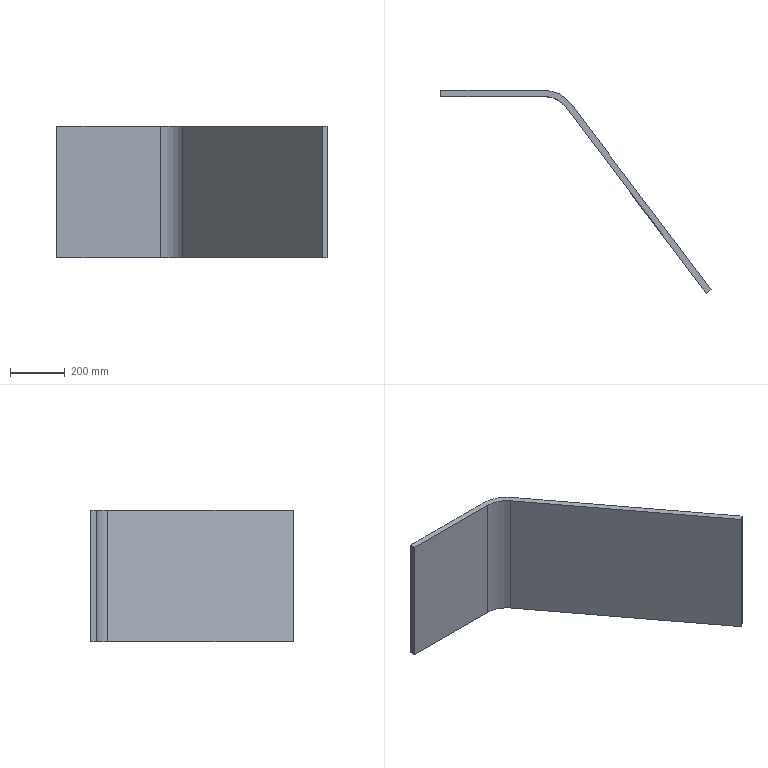Part | NX | features 底座(默认<按焊接>) 2 | 1 solid | 10 faces | box 988.426 x 741.88 x 480 mm | volume 13960123 mm3 | plane 8 | cylinder 2 | commonest cylinder face diameters 200 x1 243.64 x1
STEP:
#1=CARTESIAN_POINT('',(2564.611,34.952,-412.));
#2=VERTEX_POINT('',#1);
#3=CARTESIAN_POINT('',(2052.013,715.193,-412.));
#4=VERTEX_POINT('',#3);
#5=CARTESIAN_POINT('',(3246.385,-869.792,-412.));
#6=DIRECTION('',(-0.6018,0.7986,0.));
#7=VECTOR('',#6,1000.);
#8=LINE('',#5,#7);
#9=EDGE_CURVE('',#2,#4,#8,.T.);
#10=ORIENTED_EDGE('',*,*,#9,.F.);
#11=CARTESIAN_POINT('',(2564.611,34.952,-892.));
#12=VERTEX_POINT('',#11);
#13=CARTESIAN_POINT('',(2564.611,34.952,-892.));
#14=DIRECTION('',(0.,0.,1.));
#15=VECTOR('',#14,1000.);
#16=LINE('',#13,#15);
#17=EDGE_CURVE('',#12,#2,#16,.T.);
#18=ORIENTED_EDGE('',*,*,#17,.F.);
#19=CARTESIAN_POINT('',(2052.013,715.193,-892.));
#20=VERTEX_POINT('',#19);
#21=CARTESIAN_POINT('',(3246.385,-869.792,-892.));
#22=DIRECTION('',(-0.6018,0.7986,0.));
#23=VECTOR('',#22,1000.);
#24=LINE('',#21,#23);
#25=EDGE_CURVE('',#12,#20,#24,.T.);
#26=ORIENTED_EDGE('',*,*,#25,.T.);
#27=CARTESIAN_POINT('',(2052.013,715.193,-892.));
#28=DIRECTION('',(0.,0.,1.));
#29=VECTOR('',#28,1000.);
#30=LINE('',#27,#29);
#31=EDGE_CURVE('',#20,#4,#30,.T.);
#32=ORIENTED_EDGE('',*,*,#31,.T.);
#33=EDGE_LOOP('',(#10,#18,#26,#32));
#34=FACE_BOUND('',#33,.T.);
#35=CARTESIAN_POINT('',(3246.385,-869.792,-892.));
#36=DIRECTION('',(-0.7986,-0.6018,0.));
#37=DIRECTION('',(0.6018,-0.7986,0.));
#38=AXIS2_PLACEMENT_3D('',#35,#36,#37);
#39=PLANE('',#38);
#40=ADVANCED_FACE('',(#34),#39,.F.);
#41=CARTESIAN_POINT('',(1954.723,763.7,-412.));
#42=VERTEX_POINT('',#41);
#43=CARTESIAN_POINT('',(1954.723,641.88,-412.));
#44=DIRECTION('',(0.,0.,1.));
#45=DIRECTION('',(1.,0.,0.));
#46=AXIS2_PLACEMENT_3D('',#43,#44,#45);
#47=CIRCLE('',#46,121.82);
#48=EDGE_CURVE('',#4,#42,#47,.T.);
#49=ORIENTED_EDGE('',*,*,#48,.F.);
#50=ORIENTED_EDGE('',*,*,#31,.F.);
#51=CARTESIAN_POINT('',(1954.723,763.7,-892.));
#52=VERTEX_POINT('',#51);
#53=CARTESIAN_POINT('',(1954.723,641.88,-892.));
#54=DIRECTION('',(0.,0.,1.));
#55=DIRECTION('',(1.,0.,0.));
#56=AXIS2_PLACEMENT_3D('',#53,#54,#55);
#57=CIRCLE('',#56,121.82);
#58=EDGE_CURVE('',#20,#52,#57,.T.);
#59=ORIENTED_EDGE('',*,*,#58,.T.);
#60=CARTESIAN_POINT('',(1954.723,763.7,-892.));
#61=DIRECTION('',(0.,0.,1.));
#62=VECTOR('',#61,1000.);
#63=LINE('',#60,#62);
#64=EDGE_CURVE('',#52,#42,#63,.T.);
#65=ORIENTED_EDGE('',*,*,#64,.T.);
#66=EDGE_LOOP('',(#49,#50,#59,#65));
#67=FACE_BOUND('',#66,.T.);
#68=CARTESIAN_POINT('',(1954.723,641.88,-892.));
#69=DIRECTION('',(0.,0.,1.));
#70=DIRECTION('',(-1.,0.,0.));
#71=AXIS2_PLACEMENT_3D('',#68,#69,#70);
#72=CYLINDRICAL_SURFACE('',#71,121.82);
#73=ADVANCED_FACE('',(#67),#72,.T.);
#74=CARTESIAN_POINT('',(1576.185,763.7,-412.));
#75=VERTEX_POINT('',#74);
#76=CARTESIAN_POINT('',(1250.85,763.7,-412.));
#77=DIRECTION('',(1.,0.,0.));
#78=VECTOR('',#77,1000.);
#79=LINE('',#76,#78);
#80=EDGE_CURVE('',#75,#42,#79,.T.);
#81=ORIENTED_EDGE('',*,*,#80,.T.);
#82=ORIENTED_EDGE('',*,*,#64,.F.);
#83=CARTESIAN_POINT('',(1576.185,763.7,-892.));
#84=VERTEX_POINT('',#83);
#85=CARTESIAN_POINT('',(1250.85,763.7,-892.));
#86=DIRECTION('',(1.,0.,0.));
#87=VECTOR('',#86,1000.);
#88=LINE('',#85,#87);
#89=EDGE_CURVE('',#84,#52,#88,.T.);
#90=ORIENTED_EDGE('',*,*,#89,.F.);
#91=CARTESIAN_POINT('',(1576.185,763.7,-892.));
#92=DIRECTION('',(0.,0.,1.));
#93=VECTOR('',#92,1000.);
#94=LINE('',#91,#93);
#95=EDGE_CURVE('',#84,#75,#94,.T.);
#96=ORIENTED_EDGE('',*,*,#95,.T.);
#97=EDGE_LOOP('',(#81,#82,#90,#96));
#98=FACE_BOUND('',#97,.T.);
#99=CARTESIAN_POINT('',(1250.85,763.7,-892.));
#100=DIRECTION('',(0.,1.,0.));
#101=DIRECTION('',(0.,0.,-1.));
#102=AXIS2_PLACEMENT_3D('',#99,#100,#101);
#103=PLANE('',#102);
#104=ADVANCED_FACE('',(#98),#103,.T.);
#105=CARTESIAN_POINT('',(1576.185,741.88,-412.));
#106=VERTEX_POINT('',#105);
#107=CARTESIAN_POINT('',(1576.185,-2373.536,-412.));
#108=DIRECTION('',(0.,-1.,0.));
#109=VECTOR('',#108,1000.);
#110=LINE('',#107,#109);
#111=EDGE_CURVE('',#75,#106,#110,.T.);
#112=ORIENTED_EDGE('',*,*,#111,.F.);
#113=ORIENTED_EDGE('',*,*,#95,.F.);
#114=CARTESIAN_POINT('',(1576.185,741.88,-892.));
#115=VERTEX_POINT('',#114);
#116=CARTESIAN_POINT('',(1576.185,-2373.536,-892.));
#117=DIRECTION('',(0.,-1.,0.));
#118=VECTOR('',#117,1000.);
#119=LINE('',#116,#118);
#120=EDGE_CURVE('',#84,#115,#119,.T.);
#121=ORIENTED_EDGE('',*,*,#120,.T.);
#122=CARTESIAN_POINT('',(1576.185,741.88,-892.));
#123=DIRECTION('',(0.,0.,1.));
#124=VECTOR('',#123,1000.);
#125=LINE('',#122,#124);
#126=EDGE_CURVE('',#115,#106,#125,.T.);
#127=ORIENTED_EDGE('',*,*,#126,.T.);
#128=EDGE_LOOP('',(#112,#113,#121,#127));
#129=FACE_BOUND('',#128,.T.);
#130=CARTESIAN_POINT('',(1576.185,-2373.536,-892.));
#131=DIRECTION('',(1.,0.,0.));
#132=DIRECTION('',(0.,0.,1.));
#133=AXIS2_PLACEMENT_3D('',#130,#131,#132);
#134=PLANE('',#133);
#135=ADVANCED_FACE('',(#129),#134,.F.);
#136=CARTESIAN_POINT('',(1954.723,741.88,-412.));
#137=VERTEX_POINT('',#136);
#138=CARTESIAN_POINT('',(1250.85,741.88,-412.));
#139=DIRECTION('',(1.,0.,0.));
#140=VECTOR('',#139,1000.);
#141=LINE('',#138,#140);
#142=EDGE_CURVE('',#106,#137,#141,.T.);
#143=ORIENTED_EDGE('',*,*,#142,.F.);
#144=ORIENTED_EDGE('',*,*,#126,.F.);
#145=CARTESIAN_POINT('',(1954.723,741.88,-892.));
#146=VERTEX_POINT('',#145);
#147=CARTESIAN_POINT('',(1250.85,741.88,-892.));
#148=DIRECTION('',(1.,0.,0.));
#149=VECTOR('',#148,1000.);
#150=LINE('',#147,#149);
#151=EDGE_CURVE('',#115,#146,#150,.T.);
#152=ORIENTED_EDGE('',*,*,#151,.T.);
#153=CARTESIAN_POINT('',(1954.723,741.88,-892.));
#154=DIRECTION('',(0.,0.,1.));
#155=VECTOR('',#154,1000.);
#156=LINE('',#153,#155);
#157=EDGE_CURVE('',#146,#137,#156,.T.);
#158=ORIENTED_EDGE('',*,*,#157,.T.);
#159=EDGE_LOOP('',(#143,#144,#152,#158));
#160=FACE_BOUND('',#159,.T.);
#161=CARTESIAN_POINT('',(1250.85,741.88,-892.));
#162=DIRECTION('',(0.,1.,0.));
#163=DIRECTION('',(-1.,0.,0.));
#164=AXIS2_PLACEMENT_3D('',#161,#162,#163);
#165=PLANE('',#164);
#166=ADVANCED_FACE('',(#160),#165,.F.);
#167=CARTESIAN_POINT('',(2034.586,702.062,-412.));
#168=VERTEX_POINT('',#167);
#169=CARTESIAN_POINT('',(1954.723,641.88,-412.));
#170=DIRECTION('',(0.,0.,1.));
#171=DIRECTION('',(1.,0.,0.));
#172=AXIS2_PLACEMENT_3D('',#169,#170,#171);
#173=CIRCLE('',#172,100.);
#174=EDGE_CURVE('',#168,#137,#173,.T.);
#175=ORIENTED_EDGE('',*,*,#174,.T.);
#176=ORIENTED_EDGE('',*,*,#157,.F.);
#177=CARTESIAN_POINT('',(2034.586,702.062,-892.));
#178=VERTEX_POINT('',#177);
#179=CARTESIAN_POINT('',(1954.723,641.88,-892.));
#180=DIRECTION('',(0.,0.,1.));
#181=DIRECTION('',(1.,0.,0.));
#182=AXIS2_PLACEMENT_3D('',#179,#180,#181);
#183=CIRCLE('',#182,100.);
#184=EDGE_CURVE('',#178,#146,#183,.T.);
#185=ORIENTED_EDGE('',*,*,#184,.F.);
#186=CARTESIAN_POINT('',(2034.586,702.062,-892.));
#187=DIRECTION('',(0.,0.,1.));
#188=VECTOR('',#187,1000.);
#189=LINE('',#186,#188);
#190=EDGE_CURVE('',#178,#168,#189,.T.);
#191=ORIENTED_EDGE('',*,*,#190,.T.);
#192=EDGE_LOOP('',(#175,#176,#185,#191));
#193=FACE_BOUND('',#192,.T.);
#194=CARTESIAN_POINT('',(1954.723,641.88,-892.));
#195=DIRECTION('',(0.,0.,1.));
#196=DIRECTION('',(-1.,0.,0.));
#197=AXIS2_PLACEMENT_3D('',#194,#195,#196);
#198=CYLINDRICAL_SURFACE('',#197,100.);
#199=ADVANCED_FACE('',(#193),#198,.F.);
#200=CARTESIAN_POINT('',(2547.185,21.82,-412.));
#201=VERTEX_POINT('',#200);
#202=CARTESIAN_POINT('',(3228.959,-882.924,-412.));
#203=DIRECTION('',(-0.6018,0.7986,0.));
#204=VECTOR('',#203,1000.);
#205=LINE('',#202,#204);
#206=EDGE_CURVE('',#201,#168,#205,.T.);
#207=ORIENTED_EDGE('',*,*,#206,.T.);
#208=ORIENTED_EDGE('',*,*,#190,.F.);
#209=CARTESIAN_POINT('',(2547.185,21.82,-892.));
#210=VERTEX_POINT('',#209);
#211=CARTESIAN_POINT('',(3228.959,-882.924,-892.));
#212=DIRECTION('',(-0.6018,0.7986,0.));
#213=VECTOR('',#212,1000.);
#214=LINE('',#211,#213);
#215=EDGE_CURVE('',#210,#178,#214,.T.);
#216=ORIENTED_EDGE('',*,*,#215,.F.);
#217=CARTESIAN_POINT('',(2547.185,21.82,-892.));
#218=DIRECTION('',(0.,0.,1.));
#219=VECTOR('',#218,1000.);
#220=LINE('',#217,#219);
#221=EDGE_CURVE('',#210,#201,#220,.T.);
#222=ORIENTED_EDGE('',*,*,#221,.T.);
#223=EDGE_LOOP('',(#207,#208,#216,#222));
#224=FACE_BOUND('',#223,.T.);
#225=CARTESIAN_POINT('',(3228.959,-882.924,-892.));
#226=DIRECTION('',(-0.7986,-0.6018,0.));
#227=DIRECTION('',(0.6018,-0.7986,0.));
#228=AXIS2_PLACEMENT_3D('',#225,#226,#227);
#229=PLANE('',#228);
#230=ADVANCED_FACE('',(#224),#229,.T.);
#231=CARTESIAN_POINT('',(569.076,-1468.792,-412.));
#232=DIRECTION('',(-0.7986,-0.6018,0.));
#233=VECTOR('',#232,1000.);
#234=LINE('',#231,#233);
#235=EDGE_CURVE('',#2,#201,#234,.T.);
#236=ORIENTED_EDGE('',*,*,#235,.T.);
#237=ORIENTED_EDGE('',*,*,#221,.F.);
#238=CARTESIAN_POINT('',(569.076,-1468.792,-892.));
#239=DIRECTION('',(-0.7986,-0.6018,0.));
#240=VECTOR('',#239,1000.);
#241=LINE('',#238,#240);
#242=EDGE_CURVE('',#12,#210,#241,.T.);
#243=ORIENTED_EDGE('',*,*,#242,.F.);
#244=ORIENTED_EDGE('',*,*,#17,.T.);
#245=EDGE_LOOP('',(#236,#237,#243,#244));
#246=FACE_BOUND('',#245,.T.);
#247=CARTESIAN_POINT('',(569.076,-1468.792,-892.));
#248=DIRECTION('',(0.6018,-0.7986,0.));
#249=DIRECTION('',(0.7986,0.6018,0.));
#250=AXIS2_PLACEMENT_3D('',#247,#248,#249);
#251=PLANE('',#250);
#252=ADVANCED_FACE('',(#246),#251,.T.);
#253=ORIENTED_EDGE('',*,*,#25,.F.);
#254=ORIENTED_EDGE('',*,*,#242,.T.);
#255=ORIENTED_EDGE('',*,*,#215,.T.);
#256=ORIENTED_EDGE('',*,*,#184,.T.);
#257=ORIENTED_EDGE('',*,*,#151,.F.);
#258=ORIENTED_EDGE('',*,*,#120,.F.);
#259=ORIENTED_EDGE('',*,*,#89,.T.);
#260=ORIENTED_EDGE('',*,*,#58,.F.);
#261=EDGE_LOOP('',(#253,#254,#255,#256,#257,#258,#259,#260));
#262=FACE_BOUND('',#261,.T.);
#263=CARTESIAN_POINT('',(1250.85,-2373.536,-892.));
#264=DIRECTION('',(0.,0.,-1.));
#265=DIRECTION('',(1.,0.,0.));
#266=AXIS2_PLACEMENT_3D('',#263,#264,#265);
#267=PLANE('',#266);
#268=ADVANCED_FACE('',(#262),#267,.T.);
#269=ORIENTED_EDGE('',*,*,#9,.T.);
#270=ORIENTED_EDGE('',*,*,#48,.T.);
#271=ORIENTED_EDGE('',*,*,#80,.F.);
#272=ORIENTED_EDGE('',*,*,#111,.T.);
#273=ORIENTED_EDGE('',*,*,#142,.T.);
#274=ORIENTED_EDGE('',*,*,#174,.F.);
#275=ORIENTED_EDGE('',*,*,#206,.F.);
#276=ORIENTED_EDGE('',*,*,#235,.F.);
#277=EDGE_LOOP('',(#269,#270,#271,#272,#273,#274,#275,#276));
#278=FACE_BOUND('',#277,.T.);
#279=CARTESIAN_POINT('',(1250.85,-2373.536,-412.));
#280=DIRECTION('',(0.,0.,-1.));
#281=DIRECTION('',(1.,0.,0.));
#282=AXIS2_PLACEMENT_3D('',#279,#280,#281);
#283=PLANE('',#282);
#284=ADVANCED_FACE('',(#278),#283,.F.);
#285=CLOSED_SHELL('',(#40,#73,#104,#135,#166,#199,#230,#252,#268,#284));
#286=MANIFOLD_SOLID_BREP('',#285);
#287=(LENGTH_UNIT()NAMED_UNIT(*)SI_UNIT(.MILLI.,.METRE.));
#288=UNCERTAINTY_MEASURE_WITH_UNIT(LENGTH_MEASURE(0.00001),#287,'','');
#289=(NAMED_UNIT(*)PLANE_ANGLE_UNIT()SI_UNIT($,.RADIAN.));
#290=(NAMED_UNIT(*)SI_UNIT($,.STERADIAN.)SOLID_ANGLE_UNIT());
#291=(GEOMETRIC_REPRESENTATION_CONTEXT(3)GLOBAL_UNCERTAINTY_ASSIGNED_CONTEXT((#288))GLOBAL_UNIT_ASSIGNED_CONTEXT((#287,#289,#290))REPRESENTATION_CONTEXT('',''));
#292=ADVANCED_BREP_SHAPE_REPRESENTATION('',(#286),#291);